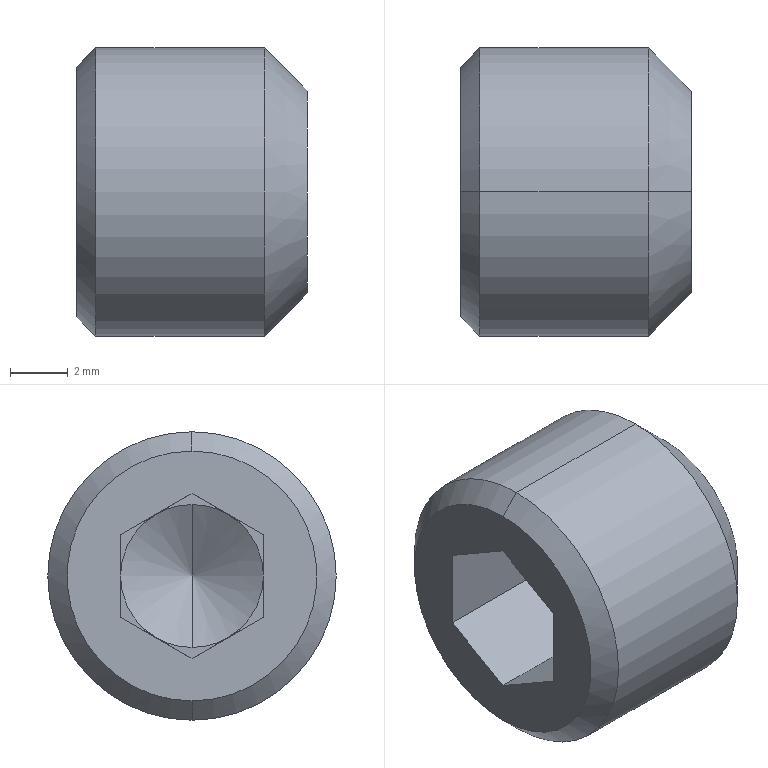Part | STEP file | 1 solid | 22 faces | box 8 x 10 x 10 mm | volume 495.582 mm3 | plane 14 | cone 6 | cylinder 2 | commonest cylinder face diameters 10 x2
STEP:
#1=CARTESIAN_POINT('',(0.,0.,0.));
#2=DIRECTION('',(0.,0.,1.));
#3=DIRECTION('',(1.,0.,0.));
#4=AXIS2_PLACEMENT_3D('',#1,#2,#3);
#5=CARTESIAN_POINT('',(4.,2.477,0.));
#6=VERTEX_POINT('',#5);
#7=CARTESIAN_POINT('',(4.,2.477,-1.43));
#8=VERTEX_POINT('',#7);
#9=CARTESIAN_POINT('',(4.,2.477,-1.43));
#10=DIRECTION('',(0.,0.,-1.));
#11=VECTOR('',#10,1.);
#12=LINE('',#9,#11);
#13=CARTESIAN_POINT('',(4.,-2.477,-1.43));
#14=DIRECTION('',(-1.,0.,0.));
#15=DIRECTION('',(0.,0.,1.));
#16=AXIS2_PLACEMENT_3D('',#13,#14,#15);
#17=PLANE('',#16);
#18=CARTESIAN_POINT('',(0.,4.954));
#19=DIRECTION('',(-1.,0.));
#20=VECTOR('',#19,1.);
#21=LINE('',#18,#20);
#22=(GEOMETRIC_REPRESENTATION_CONTEXT(2)PARAMETRIC_REPRESENTATION_CONTEXT()REPRESENTATION_CONTEXT('',''));
#23=DEFINITIONAL_REPRESENTATION('',(#21),#22);
#24=PCURVE('',#17,#23);
#25=CARTESIAN_POINT('',(4.,2.477,1.43));
#26=DIRECTION('',(0.,1.,0.));
#27=DIRECTION('',(0.,0.,-1.));
#28=AXIS2_PLACEMENT_3D('',#25,#26,#27);
#29=PLANE('',#28);
#30=CARTESIAN_POINT('',(2.86,0.));
#31=DIRECTION('',(1.,0.));
#32=VECTOR('',#31,1.);
#33=LINE('',#30,#32);
#34=(GEOMETRIC_REPRESENTATION_CONTEXT(2)PARAMETRIC_REPRESENTATION_CONTEXT()REPRESENTATION_CONTEXT('',''));
#35=DEFINITIONAL_REPRESENTATION('',(#33),#34);
#36=PCURVE('',#29,#35);
#37=SURFACE_CURVE('',#12,(#24,#36),.PCURVE_S1.);
#38=EDGE_CURVE('',#6,#8,#37,.T.);
#39=ORIENTED_EDGE('',*,*,#38,.T.);
#40=CARTESIAN_POINT('',(4.,1.238,-2.145));
#41=VERTEX_POINT('',#40);
#42=CARTESIAN_POINT('',(4.,2.477,-1.43));
#43=DIRECTION('',(0.,-0.866,-0.5));
#44=VECTOR('',#43,1.);
#45=LINE('',#42,#44);
#46=CARTESIAN_POINT('',(0.,4.954));
#47=DIRECTION('',(-0.5,-0.866));
#48=VECTOR('',#47,1.);
#49=LINE('',#46,#48);
#50=(GEOMETRIC_REPRESENTATION_CONTEXT(2)PARAMETRIC_REPRESENTATION_CONTEXT()REPRESENTATION_CONTEXT('',''));
#51=DEFINITIONAL_REPRESENTATION('',(#49),#50);
#52=PCURVE('',#17,#51);
#53=CARTESIAN_POINT('',(4.,2.477,-1.43));
#54=DIRECTION('',(0.,0.5,-0.866));
#55=DIRECTION('',(-1.,0.,0.));
#56=AXIS2_PLACEMENT_3D('',#53,#54,#55);
#57=PLANE('',#56);
#58=CARTESIAN_POINT('',(0.,0.));
#59=DIRECTION('',(0.,-1.));
#60=VECTOR('',#59,1.);
#61=LINE('',#58,#60);
#62=(GEOMETRIC_REPRESENTATION_CONTEXT(2)PARAMETRIC_REPRESENTATION_CONTEXT()REPRESENTATION_CONTEXT('',''));
#63=DEFINITIONAL_REPRESENTATION('',(#61),#62);
#64=PCURVE('',#57,#63);
#65=SURFACE_CURVE('',#45,(#52,#64),.PCURVE_S1.);
#66=EDGE_CURVE('',#8,#41,#65,.T.);
#67=ORIENTED_EDGE('',*,*,#66,.T.);
#68=CARTESIAN_POINT('',(4.,0.,0.));
#69=DIRECTION('',(1.,0.,0.));
#70=DIRECTION('',(0.,0.,1.));
#71=AXIS2_PLACEMENT_3D('',#68,#69,#70);
#72=CIRCLE('',#71,2.477);
#73=CARTESIAN_POINT('',(3.907,2.477));
#74=CARTESIAN_POINT('',(3.907,-1.813));
#75=CARTESIAN_POINT('',(0.1916,0.3318));
#76=CARTESIAN_POINT('',(-3.524,2.477));
#77=CARTESIAN_POINT('',(0.1916,4.622));
#78=CARTESIAN_POINT('',(3.907,6.767));
#79=CARTESIAN_POINT('',(3.907,2.477));
#80=(BOUNDED_CURVE()B_SPLINE_CURVE(2,(#73,#74,#75,#76,#77,#78,#79),.UNSPECIFIED.,.T.,.F.)B_SPLINE_CURVE_WITH_KNOTS((1,2,2,2,2,1),(-2.094,0.,2.094,4.189,6.283,8.378),.UNSPECIFIED.)CURVE()GEOMETRIC_REPRESENTATION_ITEM()RATIONAL_B_SPLINE_CURVE((1.,0.5,1.,0.5,1.,0.5,1.))REPRESENTATION_ITEM(''));
#81=(GEOMETRIC_REPRESENTATION_CONTEXT(2)PARAMETRIC_REPRESENTATION_CONTEXT()REPRESENTATION_CONTEXT('',''));
#82=DEFINITIONAL_REPRESENTATION('',(#80),#81);
#83=PCURVE('',#17,#82);
#84=CARTESIAN_POINT('',(4.,0.,0.));
#85=DIRECTION('',(-1.,0.,0.));
#86=DIRECTION('',(0.,0.,1.));
#87=AXIS2_PLACEMENT_3D('',#84,#85,#86);
#88=CONICAL_SURFACE('',#87,2.477,1.047);
#89=CARTESIAN_POINT('',(6.283,0.));
#90=DIRECTION('',(-1.,0.));
#91=VECTOR('',#90,1.);
#92=LINE('',#89,#91);
#93=(GEOMETRIC_REPRESENTATION_CONTEXT(2)PARAMETRIC_REPRESENTATION_CONTEXT()REPRESENTATION_CONTEXT('',''));
#94=DEFINITIONAL_REPRESENTATION('',(#92),#93);
#95=PCURVE('',#88,#94);
#96=SURFACE_CURVE('',#72,(#83,#95),.PCURVE_S1.);
#97=EDGE_CURVE('',#41,#6,#96,.T.);
#98=ORIENTED_EDGE('',*,*,#97,.T.);
#99=EDGE_LOOP('',(#39,#67,#98));
#100=FACE_BOUND('',#99,.T.);
#101=ADVANCED_FACE('',(#100),#17,.T.);
#102=CARTESIAN_POINT('',(4.,1.238,2.145));
#103=VERTEX_POINT('',#102);
#104=CARTESIAN_POINT('',(4.,2.477,1.43));
#105=VERTEX_POINT('',#104);
#106=CARTESIAN_POINT('',(4.,1.238,2.145));
#107=DIRECTION('',(0.,0.866,-0.5));
#108=VECTOR('',#107,1.);
#109=LINE('',#106,#108);
#110=CARTESIAN_POINT('',(4.,-2.477,-1.43));
#111=DIRECTION('',(-1.,0.,0.));
#112=DIRECTION('',(0.,0.,1.));
#113=AXIS2_PLACEMENT_3D('',#110,#111,#112);
#114=PLANE('',#113);
#115=CARTESIAN_POINT('',(3.575,3.715));
#116=DIRECTION('',(-0.5,0.866));
#117=VECTOR('',#116,1.);
#118=LINE('',#115,#117);
#119=(GEOMETRIC_REPRESENTATION_CONTEXT(2)PARAMETRIC_REPRESENTATION_CONTEXT()REPRESENTATION_CONTEXT('',''));
#120=DEFINITIONAL_REPRESENTATION('',(#118),#119);
#121=PCURVE('',#114,#120);
#122=CARTESIAN_POINT('',(4.,0.,2.86));
#123=DIRECTION('',(0.,0.5,0.866));
#124=DIRECTION('',(1.,0.,0.));
#125=AXIS2_PLACEMENT_3D('',#122,#123,#124);
#126=PLANE('',#125);
#127=CARTESIAN_POINT('',(0.,1.43));
#128=DIRECTION('',(0.,1.));
#129=VECTOR('',#128,1.);
#130=LINE('',#127,#129);
#131=(GEOMETRIC_REPRESENTATION_CONTEXT(2)PARAMETRIC_REPRESENTATION_CONTEXT()REPRESENTATION_CONTEXT('',''));
#132=DEFINITIONAL_REPRESENTATION('',(#130),#131);
#133=PCURVE('',#126,#132);
#134=SURFACE_CURVE('',#109,(#121,#133),.PCURVE_S1.);
#135=EDGE_CURVE('',#103,#105,#134,.T.);
#136=ORIENTED_EDGE('',*,*,#135,.T.);
#137=CARTESIAN_POINT('',(4.,2.477,-1.43));
#138=DIRECTION('',(0.,0.,-1.));
#139=VECTOR('',#138,1.);
#140=LINE('',#137,#139);
#141=CARTESIAN_POINT('',(0.,4.954));
#142=DIRECTION('',(-1.,0.));
#143=VECTOR('',#142,1.);
#144=LINE('',#141,#143);
#145=(GEOMETRIC_REPRESENTATION_CONTEXT(2)PARAMETRIC_REPRESENTATION_CONTEXT()REPRESENTATION_CONTEXT('',''));
#146=DEFINITIONAL_REPRESENTATION('',(#144),#145);
#147=PCURVE('',#114,#146);
#148=CARTESIAN_POINT('',(2.86,0.));
#149=DIRECTION('',(1.,0.));
#150=VECTOR('',#149,1.);
#151=LINE('',#148,#150);
#152=(GEOMETRIC_REPRESENTATION_CONTEXT(2)PARAMETRIC_REPRESENTATION_CONTEXT()REPRESENTATION_CONTEXT('',''));
#153=DEFINITIONAL_REPRESENTATION('',(#151),#152);
#154=PCURVE('',#29,#153);
#155=SURFACE_CURVE('',#140,(#147,#154),.PCURVE_S1.);
#156=EDGE_CURVE('',#105,#6,#155,.T.);
#157=ORIENTED_EDGE('',*,*,#156,.T.);
#158=CARTESIAN_POINT('',(4.,0.,0.));
#159=DIRECTION('',(1.,0.,0.));
#160=DIRECTION('',(0.,0.,1.));
#161=AXIS2_PLACEMENT_3D('',#158,#159,#160);
#162=CIRCLE('',#161,2.477);
#163=CARTESIAN_POINT('',(3.907,2.477));
#164=CARTESIAN_POINT('',(3.907,-1.813));
#165=CARTESIAN_POINT('',(0.1916,0.3318));
#166=CARTESIAN_POINT('',(-3.524,2.477));
#167=CARTESIAN_POINT('',(0.1916,4.622));
#168=CARTESIAN_POINT('',(3.907,6.767));
#169=CARTESIAN_POINT('',(3.907,2.477));
#170=(BOUNDED_CURVE()B_SPLINE_CURVE(2,(#163,#164,#165,#166,#167,#168,#169),.UNSPECIFIED.,.T.,.F.)B_SPLINE_CURVE_WITH_KNOTS((1,2,2,2,2,1),(-2.094,0.,2.094,4.189,6.283,8.378),.UNSPECIFIED.)CURVE()GEOMETRIC_REPRESENTATION_ITEM()RATIONAL_B_SPLINE_CURVE((1.,0.5,1.,0.5,1.,0.5,1.))REPRESENTATION_ITEM(''));
#171=(GEOMETRIC_REPRESENTATION_CONTEXT(2)PARAMETRIC_REPRESENTATION_CONTEXT()REPRESENTATION_CONTEXT('',''));
#172=DEFINITIONAL_REPRESENTATION('',(#170),#171);
#173=PCURVE('',#114,#172);
#174=CARTESIAN_POINT('',(6.283,0.));
#175=DIRECTION('',(-1.,0.));
#176=VECTOR('',#175,1.);
#177=LINE('',#174,#176);
#178=(GEOMETRIC_REPRESENTATION_CONTEXT(2)PARAMETRIC_REPRESENTATION_CONTEXT()REPRESENTATION_CONTEXT('',''));
#179=DEFINITIONAL_REPRESENTATION('',(#177),#178);
#180=PCURVE('',#88,#179);
#181=SURFACE_CURVE('',#162,(#173,#180),.PCURVE_S1.);
#182=EDGE_CURVE('',#6,#103,#181,.T.);
#183=ORIENTED_EDGE('',*,*,#182,.T.);
#184=EDGE_LOOP('',(#136,#157,#183));
#185=FACE_BOUND('',#184,.T.);
#186=ADVANCED_FACE('',(#185),#114,.T.);
#187=CARTESIAN_POINT('',(4.,-1.238,-2.145));
#188=VERTEX_POINT('',#187);
#189=CARTESIAN_POINT('',(4.,-2.477,-1.43));
#190=VERTEX_POINT('',#189);
#191=CARTESIAN_POINT('',(4.,-1.238,-2.145));
#192=DIRECTION('',(0.,-0.866,0.5));
#193=VECTOR('',#192,1.);
#194=LINE('',#191,#193);
#195=CARTESIAN_POINT('',(4.,-2.477,-1.43));
#196=DIRECTION('',(-1.,0.,0.));
#197=DIRECTION('',(0.,0.,1.));
#198=AXIS2_PLACEMENT_3D('',#195,#196,#197);
#199=PLANE('',#198);
#200=CARTESIAN_POINT('',(-0.715,1.238));
#201=DIRECTION('',(0.5,-0.866));
#202=VECTOR('',#201,1.);
#203=LINE('',#200,#202);
#204=(GEOMETRIC_REPRESENTATION_CONTEXT(2)PARAMETRIC_REPRESENTATION_CONTEXT()REPRESENTATION_CONTEXT('',''));
#205=DEFINITIONAL_REPRESENTATION('',(#203),#204);
#206=PCURVE('',#199,#205);
#207=CARTESIAN_POINT('',(4.,0.,-2.86));
#208=DIRECTION('',(0.,-0.5,-0.866));
#209=DIRECTION('',(0.,-0.866,0.5));
#210=AXIS2_PLACEMENT_3D('',#207,#208,#209);
#211=PLANE('',#210);
#212=CARTESIAN_POINT('',(1.43,0.));
#213=DIRECTION('',(1.,0.));
#214=VECTOR('',#213,1.);
#215=LINE('',#212,#214);
#216=(GEOMETRIC_REPRESENTATION_CONTEXT(2)PARAMETRIC_REPRESENTATION_CONTEXT()REPRESENTATION_CONTEXT('',''));
#217=DEFINITIONAL_REPRESENTATION('',(#215),#216);
#218=PCURVE('',#211,#217);
#219=SURFACE_CURVE('',#194,(#206,#218),.PCURVE_S1.);
#220=EDGE_CURVE('',#188,#190,#219,.T.);
#221=ORIENTED_EDGE('',*,*,#220,.T.);
#222=CARTESIAN_POINT('',(4.,-2.477,0.));
#223=VERTEX_POINT('',#222);
#224=CARTESIAN_POINT('',(4.,-2.477,-1.43));
#225=DIRECTION('',(0.,0.,1.));
#226=VECTOR('',#225,1.);
#227=LINE('',#224,#226);
#228=CARTESIAN_POINT('',(0.,0.));
#229=DIRECTION('',(1.,0.));
#230=VECTOR('',#229,1.);
#231=LINE('',#228,#230);
#232=(GEOMETRIC_REPRESENTATION_CONTEXT(2)PARAMETRIC_REPRESENTATION_CONTEXT()REPRESENTATION_CONTEXT('',''));
#233=DEFINITIONAL_REPRESENTATION('',(#231),#232);
#234=PCURVE('',#199,#233);
#235=CARTESIAN_POINT('',(4.,-2.477,-1.43));
#236=DIRECTION('',(0.,-1.,0.));
#237=DIRECTION('',(-1.,0.,0.));
#238=AXIS2_PLACEMENT_3D('',#235,#236,#237);
#239=PLANE('',#238);
#240=CARTESIAN_POINT('',(0.,0.));
#241=DIRECTION('',(0.,-1.));
#242=VECTOR('',#241,1.);
#243=LINE('',#240,#242);
#244=(GEOMETRIC_REPRESENTATION_CONTEXT(2)PARAMETRIC_REPRESENTATION_CONTEXT()REPRESENTATION_CONTEXT('',''));
#245=DEFINITIONAL_REPRESENTATION('',(#243),#244);
#246=PCURVE('',#239,#245);
#247=SURFACE_CURVE('',#227,(#234,#246),.PCURVE_S1.);
#248=EDGE_CURVE('',#190,#223,#247,.T.);
#249=ORIENTED_EDGE('',*,*,#248,.T.);
#250=CARTESIAN_POINT('',(4.,0.,0.));
#251=DIRECTION('',(1.,0.,0.));
#252=DIRECTION('',(0.,0.,1.));
#253=AXIS2_PLACEMENT_3D('',#250,#251,#252);
#254=CIRCLE('',#253,2.477);
#255=CARTESIAN_POINT('',(3.907,2.477));
#256=CARTESIAN_POINT('',(3.907,-1.813));
#257=CARTESIAN_POINT('',(0.1916,0.3318));
#258=CARTESIAN_POINT('',(-3.524,2.477));
#259=CARTESIAN_POINT('',(0.1916,4.622));
#260=CARTESIAN_POINT('',(3.907,6.767));
#261=CARTESIAN_POINT('',(3.907,2.477));
#262=(BOUNDED_CURVE()B_SPLINE_CURVE(2,(#255,#256,#257,#258,#259,#260,#261),.UNSPECIFIED.,.T.,.F.)B_SPLINE_CURVE_WITH_KNOTS((1,2,2,2,2,1),(-2.094,0.,2.094,4.189,6.283,8.378),.UNSPECIFIED.)CURVE()GEOMETRIC_REPRESENTATION_ITEM()RATIONAL_B_SPLINE_CURVE((1.,0.5,1.,0.5,1.,0.5,1.))REPRESENTATION_ITEM(''));
#263=(GEOMETRIC_REPRESENTATION_CONTEXT(2)PARAMETRIC_REPRESENTATION_CONTEXT()REPRESENTATION_CONTEXT('',''));
#264=DEFINITIONAL_REPRESENTATION('',(#262),#263);
#265=PCURVE('',#199,#264);
#266=CARTESIAN_POINT('',(4.,0.,0.));
#267=DIRECTION('',(-1.,0.,0.));
#268=DIRECTION('',(0.,0.,1.));
#269=AXIS2_PLACEMENT_3D('',#266,#267,#268);
#270=CONICAL_SURFACE('',#269,2.477,1.047);
#271=CARTESIAN_POINT('',(6.283,0.));
#272=DIRECTION('',(-1.,0.));
#273=VECTOR('',#272,1.);
#274=LINE('',#271,#273);
#275=(GEOMETRIC_REPRESENTATION_CONTEXT(2)PARAMETRIC_REPRESENTATION_CONTEXT()REPRESENTATION_CONTEXT('',''));
#276=DEFINITIONAL_REPRESENTATION('',(#274),#275);
#277=PCURVE('',#270,#276);
#278=SURFACE_CURVE('',#254,(#265,#277),.PCURVE_S1.);
#279=EDGE_CURVE('',#223,#188,#278,.T.);
#280=ORIENTED_EDGE('',*,*,#279,.T.);
#281=EDGE_LOOP('',(#221,#249,#280));
#282=FACE_BOUND('',#281,.T.);
#283=ADVANCED_FACE('',(#282),#199,.T.);
#284=CARTESIAN_POINT('',(4.,0.,-2.477));
#285=VERTEX_POINT('',#284);
#286=CARTESIAN_POINT('',(4.,0.,0.));
#287=DIRECTION('',(1.,0.,0.));
#288=DIRECTION('',(0.,0.,1.));
#289=AXIS2_PLACEMENT_3D('',#286,#287,#288);
#290=CIRCLE('',#289,2.477);
#291=CARTESIAN_POINT('',(6.283,0.));
#292=DIRECTION('',(-1.,0.));
#293=VECTOR('',#292,1.);
#294=LINE('',#291,#293);
#295=(GEOMETRIC_REPRESENTATION_CONTEXT(2)PARAMETRIC_REPRESENTATION_CONTEXT()REPRESENTATION_CONTEXT('',''));
#296=DEFINITIONAL_REPRESENTATION('',(#294),#295);
#297=PCURVE('',#88,#296);
#298=CARTESIAN_POINT('',(4.,-2.477,-1.43));
#299=DIRECTION('',(-1.,0.,0.));
#300=DIRECTION('',(0.,0.,1.));
#301=AXIS2_PLACEMENT_3D('',#298,#299,#300);
#302=PLANE('',#301);
#303=CARTESIAN_POINT('',(3.907,2.477));
#304=CARTESIAN_POINT('',(3.907,-1.813));
#305=CARTESIAN_POINT('',(0.1916,0.3318));
#306=CARTESIAN_POINT('',(-3.524,2.477));
#307=CARTESIAN_POINT('',(0.1916,4.622));
#308=CARTESIAN_POINT('',(3.907,6.767));
#309=CARTESIAN_POINT('',(3.907,2.477));
#310=(BOUNDED_CURVE()B_SPLINE_CURVE(2,(#303,#304,#305,#306,#307,#308,#309),.UNSPECIFIED.,.T.,.F.)B_SPLINE_CURVE_WITH_KNOTS((1,2,2,2,2,1),(-2.094,0.,2.094,4.189,6.283,8.378),.UNSPECIFIED.)CURVE()GEOMETRIC_REPRESENTATION_ITEM()RATIONAL_B_SPLINE_CURVE((1.,0.5,1.,0.5,1.,0.5,1.))REPRESENTATION_ITEM(''));
#311=(GEOMETRIC_REPRESENTATION_CONTEXT(2)PARAMETRIC_REPRESENTATION_CONTEXT()REPRESENTATION_CONTEXT('',''));
#312=DEFINITIONAL_REPRESENTATION('',(#310),#311);
#313=PCURVE('',#302,#312);
#314=SURFACE_CURVE('',#290,(#297,#313),.PCURVE_S1.);
#315=EDGE_CURVE('',#285,#41,#314,.T.);
#316=ORIENTED_EDGE('',*,*,#315,.T.);
#317=ORIENTED_EDGE('',*,*,#97,.T.);
#318=ORIENTED_EDGE('',*,*,#182,.T.);
#319=CARTESIAN_POINT('',(4.,0.,2.477));
#320=VERTEX_POINT('',#319);
#321=CARTESIAN_POINT('',(4.,0.,0.));
#322=DIRECTION('',(1.,0.,0.));
#323=DIRECTION('',(0.,0.,1.));
#324=AXIS2_PLACEMENT_3D('',#321,#322,#323);
#325=CIRCLE('',#324,2.477);
#326=CARTESIAN_POINT('',(6.283,0.));
#327=DIRECTION('',(-1.,0.));
#328=VECTOR('',#327,1.);
#329=LINE('',#326,#328);
#330=(GEOMETRIC_REPRESENTATION_CONTEXT(2)PARAMETRIC_REPRESENTATION_CONTEXT()REPRESENTATION_CONTEXT('',''));
#331=DEFINITIONAL_REPRESENTATION('',(#329),#330);
#332=PCURVE('',#88,#331);
#333=CARTESIAN_POINT('',(4.,-2.477,-1.43));
#334=DIRECTION('',(-1.,0.,0.));
#335=DIRECTION('',(0.,0.,1.));
#336=AXIS2_PLACEMENT_3D('',#333,#334,#335);
#337=PLANE('',#336);
#338=CARTESIAN_POINT('',(3.907,2.477));
#339=CARTESIAN_POINT('',(3.907,-1.813));
#340=CARTESIAN_POINT('',(0.1916,0.3318));
#341=CARTESIAN_POINT('',(-3.524,2.477));
#342=CARTESIAN_POINT('',(0.1916,4.622));
#343=CARTESIAN_POINT('',(3.907,6.767));
#344=CARTESIAN_POINT('',(3.907,2.477));
#345=(BOUNDED_CURVE()B_SPLINE_CURVE(2,(#338,#339,#340,#341,#342,#343,#344),.UNSPECIFIED.,.T.,.F.)B_SPLINE_CURVE_WITH_KNOTS((1,2,2,2,2,1),(-2.094,0.,2.094,4.189,6.283,8.378),.UNSPECIFIED.)CURVE()GEOMETRIC_REPRESENTATION_ITEM()RATIONAL_B_SPLINE_CURVE((1.,0.5,1.,0.5,1.,0.5,1.))REPRESENTATION_ITEM(''));
#346=(GEOMETRIC_REPRESENTATION_CONTEXT(2)PARAMETRIC_REPRESENTATION_CONTEXT()REPRESENTATION_CONTEXT('',''));
#347=DEFINITIONAL_REPRESENTATION('',(#345),#346);
#348=PCURVE('',#337,#347);
#349=SURFACE_CURVE('',#325,(#332,#348),.PCURVE_S1.);
#350=EDGE_CURVE('',#103,#320,#349,.T.);
#351=ORIENTED_EDGE('',*,*,#350,.T.);
#352=CARTESIAN_POINT('',(5.43,0.,0.));
#353=VERTEX_POINT('',#352);
#354=CARTESIAN_POINT('',(4.,0.,2.477));
#355=DIRECTION('',(-0.5,0.,0.866));
#356=VECTOR('',#355,1.);
#357=LINE('',#354,#356);
#358=CARTESIAN_POINT('',(0.,0.));
#359=DIRECTION('',(0.,1.));
#360=VECTOR('',#359,1.);
#361=LINE('',#358,#360);
#362=(GEOMETRIC_REPRESENTATION_CONTEXT(2)PARAMETRIC_REPRESENTATION_CONTEXT()REPRESENTATION_CONTEXT('',''));
#363=DEFINITIONAL_REPRESENTATION('',(#361),#362);
#364=PCURVE('',#88,#363);
#365=CARTESIAN_POINT('',(6.283,0.));
#366=DIRECTION('',(0.,1.));
#367=VECTOR('',#366,1.);
#368=LINE('',#365,#367);
#369=(GEOMETRIC_REPRESENTATION_CONTEXT(2)PARAMETRIC_REPRESENTATION_CONTEXT()REPRESENTATION_CONTEXT('',''));
#370=DEFINITIONAL_REPRESENTATION('',(#368),#369);
#371=PCURVE('',#270,#370);
#372=SURFACE_CURVE('',#357,(#364,#371),.PCURVE_S1.);
#373=EDGE_CURVE('',#353,#320,#372,.T.);
#374=ORIENTED_EDGE('',*,*,#373,.F.);
#375=CARTESIAN_POINT('',(4.,0.,-2.477));
#376=DIRECTION('',(-0.5,0.,-0.866));
#377=VECTOR('',#376,1.);
#378=LINE('',#375,#377);
#379=CARTESIAN_POINT('',(3.142,0.));
#380=DIRECTION('',(0.,1.));
#381=VECTOR('',#380,1.);
#382=LINE('',#379,#381);
#383=(GEOMETRIC_REPRESENTATION_CONTEXT(2)PARAMETRIC_REPRESENTATION_CONTEXT()REPRESENTATION_CONTEXT('',''));
#384=DEFINITIONAL_REPRESENTATION('',(#382),#383);
#385=PCURVE('',#88,#384);
#386=CARTESIAN_POINT('',(3.142,0.));
#387=DIRECTION('',(0.,1.));
#388=VECTOR('',#387,1.);
#389=LINE('',#386,#388);
#390=(GEOMETRIC_REPRESENTATION_CONTEXT(2)PARAMETRIC_REPRESENTATION_CONTEXT()REPRESENTATION_CONTEXT('',''));
#391=DEFINITIONAL_REPRESENTATION('',(#389),#390);
#392=PCURVE('',#270,#391);
#393=SURFACE_CURVE('',#378,(#385,#392),.PCURVE_S1.);
#394=EDGE_CURVE('',#353,#285,#393,.T.);
#395=ORIENTED_EDGE('',*,*,#394,.T.);
#396=EDGE_LOOP('',(#316,#317,#318,#351,#374,#395));
#397=FACE_BOUND('',#396,.F.);
#398=ADVANCED_FACE('',(#397),#88,.F.);
#399=CARTESIAN_POINT('',(4.,-2.477,1.43));
#400=VERTEX_POINT('',#399);
#401=CARTESIAN_POINT('',(4.,-2.477,-1.43));
#402=DIRECTION('',(0.,0.,1.));
#403=VECTOR('',#402,1.);
#404=LINE('',#401,#403);
#405=CARTESIAN_POINT('',(4.,-2.477,-1.43));
#406=DIRECTION('',(-1.,0.,0.));
#407=DIRECTION('',(0.,0.,1.));
#408=AXIS2_PLACEMENT_3D('',#405,#406,#407);
#409=PLANE('',#408);
#410=CARTESIAN_POINT('',(0.,0.));
#411=DIRECTION('',(1.,0.));
#412=VECTOR('',#411,1.);
#413=LINE('',#410,#412);
#414=(GEOMETRIC_REPRESENTATION_CONTEXT(2)PARAMETRIC_REPRESENTATION_CONTEXT()REPRESENTATION_CONTEXT('',''));
#415=DEFINITIONAL_REPRESENTATION('',(#413),#414);
#416=PCURVE('',#409,#415);
#417=CARTESIAN_POINT('',(0.,0.));
#418=DIRECTION('',(0.,-1.));
#419=VECTOR('',#418,1.);
#420=LINE('',#417,#419);
#421=(GEOMETRIC_REPRESENTATION_CONTEXT(2)PARAMETRIC_REPRESENTATION_CONTEXT()REPRESENTATION_CONTEXT('',''));
#422=DEFINITIONAL_REPRESENTATION('',(#420),#421);
#423=PCURVE('',#239,#422);
#424=SURFACE_CURVE('',#404,(#416,#423),.PCURVE_S1.);
#425=EDGE_CURVE('',#223,#400,#424,.T.);
#426=ORIENTED_EDGE('',*,*,#425,.T.);
#427=CARTESIAN_POINT('',(4.,-1.238,2.145));
#428=VERTEX_POINT('',#427);
#429=CARTESIAN_POINT('',(4.,-2.477,1.43));
#430=DIRECTION('',(0.,0.866,0.5));
#431=VECTOR('',#430,1.);
#432=LINE('',#429,#431);
#433=CARTESIAN_POINT('',(2.86,0.));
#434=DIRECTION('',(0.5,0.866));
#435=VECTOR('',#434,1.);
#436=LINE('',#433,#435);
#437=(GEOMETRIC_REPRESENTATION_CONTEXT(2)PARAMETRIC_REPRESENTATION_CONTEXT()REPRESENTATION_CONTEXT('',''));
#438=DEFINITIONAL_REPRESENTATION('',(#436),#437);
#439=PCURVE('',#409,#438);
#440=CARTESIAN_POINT('',(4.,-2.477,1.43));
#441=DIRECTION('',(0.,-0.5,0.866));
#442=DIRECTION('',(-1.,0.,0.));
#443=AXIS2_PLACEMENT_3D('',#440,#441,#442);
#444=PLANE('',#443);
#445=CARTESIAN_POINT('',(0.,0.));
#446=DIRECTION('',(0.,-1.));
#447=VECTOR('',#446,1.);
#448=LINE('',#445,#447);
#449=(GEOMETRIC_REPRESENTATION_CONTEXT(2)PARAMETRIC_REPRESENTATION_CONTEXT()REPRESENTATION_CONTEXT('',''));
#450=DEFINITIONAL_REPRESENTATION('',(#448),#449);
#451=PCURVE('',#444,#450);
#452=SURFACE_CURVE('',#432,(#439,#451),.PCURVE_S1.);
#453=EDGE_CURVE('',#400,#428,#452,.T.);
#454=ORIENTED_EDGE('',*,*,#453,.T.);
#455=CARTESIAN_POINT('',(4.,0.,0.));
#456=DIRECTION('',(1.,0.,0.));
#457=DIRECTION('',(0.,0.,1.));
#458=AXIS2_PLACEMENT_3D('',#455,#456,#457);
#459=CIRCLE('',#458,2.477);
#460=CARTESIAN_POINT('',(3.907,2.477));
#461=CARTESIAN_POINT('',(3.907,-1.813));
#462=CARTESIAN_POINT('',(0.1916,0.3318));
#463=CARTESIAN_POINT('',(-3.524,2.477));
#464=CARTESIAN_POINT('',(0.1916,4.622));
#465=CARTESIAN_POINT('',(3.907,6.767));
#466=CARTESIAN_POINT('',(3.907,2.477));
#467=(BOUNDED_CURVE()B_SPLINE_CURVE(2,(#460,#461,#462,#463,#464,#465,#466),.UNSPECIFIED.,.T.,.F.)B_SPLINE_CURVE_WITH_KNOTS((1,2,2,2,2,1),(-2.094,0.,2.094,4.189,6.283,8.378),.UNSPECIFIED.)CURVE()GEOMETRIC_REPRESENTATION_ITEM()RATIONAL_B_SPLINE_CURVE((1.,0.5,1.,0.5,1.,0.5,1.))REPRESENTATION_ITEM(''));
#468=(GEOMETRIC_REPRESENTATION_CONTEXT(2)PARAMETRIC_REPRESENTATION_CONTEXT()REPRESENTATION_CONTEXT('',''));
#469=DEFINITIONAL_REPRESENTATION('',(#467),#468);
#470=PCURVE('',#409,#469);
#471=CARTESIAN_POINT('',(6.283,0.));
#472=DIRECTION('',(-1.,0.));
#473=VECTOR('',#472,1.);
#474=LINE('',#471,#473);
#475=(GEOMETRIC_REPRESENTATION_CONTEXT(2)PARAMETRIC_REPRESENTATION_CONTEXT()REPRESENTATION_CONTEXT('',''));
#476=DEFINITIONAL_REPRESENTATION('',(#474),#475);
#477=PCURVE('',#270,#476);
#478=SURFACE_CURVE('',#459,(#470,#477),.PCURVE_S1.);
#479=EDGE_CURVE('',#428,#223,#478,.T.);
#480=ORIENTED_EDGE('',*,*,#479,.T.);
#481=EDGE_LOOP('',(#426,#454,#480));
#482=FACE_BOUND('',#481,.T.);
#483=ADVANCED_FACE('',(#482),#409,.T.);
#484=CARTESIAN_POINT('',(4.,0.,2.86));
#485=VERTEX_POINT('',#484);
#486=CARTESIAN_POINT('',(4.,0.,2.86));
#487=DIRECTION('',(0.,0.866,-0.5));
#488=VECTOR('',#487,1.);
#489=LINE('',#486,#488);
#490=CARTESIAN_POINT('',(4.29,2.477));
#491=DIRECTION('',(-0.5,0.866));
#492=VECTOR('',#491,1.);
#493=LINE('',#490,#492);
#494=(GEOMETRIC_REPRESENTATION_CONTEXT(2)PARAMETRIC_REPRESENTATION_CONTEXT()REPRESENTATION_CONTEXT('',''));
#495=DEFINITIONAL_REPRESENTATION('',(#493),#494);
#496=PCURVE('',#337,#495);
#497=CARTESIAN_POINT('',(0.,0.));
#498=DIRECTION('',(0.,1.));
#499=VECTOR('',#498,1.);
#500=LINE('',#497,#499);
#501=(GEOMETRIC_REPRESENTATION_CONTEXT(2)PARAMETRIC_REPRESENTATION_CONTEXT()REPRESENTATION_CONTEXT('',''));
#502=DEFINITIONAL_REPRESENTATION('',(#500),#501);
#503=PCURVE('',#126,#502);
#504=SURFACE_CURVE('',#489,(#496,#503),.PCURVE_S1.);
#505=EDGE_CURVE('',#485,#103,#504,.T.);
#506=ORIENTED_EDGE('',*,*,#505,.T.);
#507=ORIENTED_EDGE('',*,*,#350,.T.);
#508=CARTESIAN_POINT('',(4.,0.,0.));
#509=DIRECTION('',(1.,0.,0.));
#510=DIRECTION('',(0.,0.,1.));
#511=AXIS2_PLACEMENT_3D('',#508,#509,#510);
#512=CIRCLE('',#511,2.477);
#513=CARTESIAN_POINT('',(3.907,2.477));
#514=CARTESIAN_POINT('',(3.907,-1.813));
#515=CARTESIAN_POINT('',(0.1916,0.3318));
#516=CARTESIAN_POINT('',(-3.524,2.477));
#517=CARTESIAN_POINT('',(0.1916,4.622));
#518=CARTESIAN_POINT('',(3.907,6.767));
#519=CARTESIAN_POINT('',(3.907,2.477));
#520=(BOUNDED_CURVE()B_SPLINE_CURVE(2,(#513,#514,#515,#516,#517,#518,#519),.UNSPECIFIED.,.T.,.F.)B_SPLINE_CURVE_WITH_KNOTS((1,2,2,2,2,1),(-2.094,0.,2.094,4.189,6.283,8.378),.UNSPECIFIED.)CURVE()GEOMETRIC_REPRESENTATION_ITEM()RATIONAL_B_SPLINE_CURVE((1.,0.5,1.,0.5,1.,0.5,1.))REPRESENTATION_ITEM(''));
#521=(GEOMETRIC_REPRESENTATION_CONTEXT(2)PARAMETRIC_REPRESENTATION_CONTEXT()REPRESENTATION_CONTEXT('',''));
#522=DEFINITIONAL_REPRESENTATION('',(#520),#521);
#523=PCURVE('',#337,#522);
#524=CARTESIAN_POINT('',(6.283,0.));
#525=DIRECTION('',(-1.,0.));
#526=VECTOR('',#525,1.);
#527=LINE('',#524,#526);
#528=(GEOMETRIC_REPRESENTATION_CONTEXT(2)PARAMETRIC_REPRESENTATION_CONTEXT()REPRESENTATION_CONTEXT('',''));
#529=DEFINITIONAL_REPRESENTATION('',(#527),#528);
#530=PCURVE('',#270,#529);
#531=SURFACE_CURVE('',#512,(#523,#530),.PCURVE_S1.);
#532=EDGE_CURVE('',#320,#428,#531,.T.);
#533=ORIENTED_EDGE('',*,*,#532,.T.);
#534=CARTESIAN_POINT('',(4.,-2.477,1.43));
#535=DIRECTION('',(0.,0.866,0.5));
#536=VECTOR('',#535,1.);
#537=LINE('',#534,#536);
#538=CARTESIAN_POINT('',(2.86,0.));
#539=DIRECTION('',(0.5,0.866));
#540=VECTOR('',#539,1.);
#541=LINE('',#538,#540);
#542=(GEOMETRIC_REPRESENTATION_CONTEXT(2)PARAMETRIC_REPRESENTATION_CONTEXT()REPRESENTATION_CONTEXT('',''));
#543=DEFINITIONAL_REPRESENTATION('',(#541),#542);
#544=PCURVE('',#337,#543);
#545=CARTESIAN_POINT('',(0.,0.));
#546=DIRECTION('',(0.,-1.));
#547=VECTOR('',#546,1.);
#548=LINE('',#545,#547);
#549=(GEOMETRIC_REPRESENTATION_CONTEXT(2)PARAMETRIC_REPRESENTATION_CONTEXT()REPRESENTATION_CONTEXT('',''));
#550=DEFINITIONAL_REPRESENTATION('',(#548),#549);
#551=PCURVE('',#444,#550);
#552=SURFACE_CURVE('',#537,(#544,#551),.PCURVE_S1.);
#553=EDGE_CURVE('',#428,#485,#552,.T.);
#554=ORIENTED_EDGE('',*,*,#553,.T.);
#555=EDGE_LOOP('',(#506,#507,#533,#554));
#556=FACE_BOUND('',#555,.T.);
#557=ADVANCED_FACE('',(#556),#337,.T.);
#558=CARTESIAN_POINT('',(4.,0.,-2.86));
#559=VERTEX_POINT('',#558);
#560=CARTESIAN_POINT('',(4.,0.,-2.86));
#561=DIRECTION('',(0.,-0.866,0.5));
#562=VECTOR('',#561,1.);
#563=LINE('',#560,#562);
#564=CARTESIAN_POINT('',(-1.43,2.477));
#565=DIRECTION('',(0.5,-0.866));
#566=VECTOR('',#565,1.);
#567=LINE('',#564,#566);
#568=(GEOMETRIC_REPRESENTATION_CONTEXT(2)PARAMETRIC_REPRESENTATION_CONTEXT()REPRESENTATION_CONTEXT('',''));
#569=DEFINITIONAL_REPRESENTATION('',(#567),#568);
#570=PCURVE('',#302,#569);
#571=CARTESIAN_POINT('',(0.,0.));
#572=DIRECTION('',(1.,0.));
#573=VECTOR('',#572,1.);
#574=LINE('',#571,#573);
#575=(GEOMETRIC_REPRESENTATION_CONTEXT(2)PARAMETRIC_REPRESENTATION_CONTEXT()REPRESENTATION_CONTEXT('',''));
#576=DEFINITIONAL_REPRESENTATION('',(#574),#575);
#577=PCURVE('',#211,#576);
#578=SURFACE_CURVE('',#563,(#570,#577),.PCURVE_S1.);
#579=EDGE_CURVE('',#559,#188,#578,.T.);
#580=ORIENTED_EDGE('',*,*,#579,.T.);
#581=CARTESIAN_POINT('',(4.,0.,0.));
#582=DIRECTION('',(1.,0.,0.));
#583=DIRECTION('',(0.,0.,1.));
#584=AXIS2_PLACEMENT_3D('',#581,#582,#583);
#585=CIRCLE('',#584,2.477);
#586=CARTESIAN_POINT('',(3.907,2.477));
#587=CARTESIAN_POINT('',(3.907,-1.813));
#588=CARTESIAN_POINT('',(0.1916,0.3318));
#589=CARTESIAN_POINT('',(-3.524,2.477));
#590=CARTESIAN_POINT('',(0.1916,4.622));
#591=CARTESIAN_POINT('',(3.907,6.767));
#592=CARTESIAN_POINT('',(3.907,2.477));
#593=(BOUNDED_CURVE()B_SPLINE_CURVE(2,(#586,#587,#588,#589,#590,#591,#592),.UNSPECIFIED.,.T.,.F.)B_SPLINE_CURVE_WITH_KNOTS((1,2,2,2,2,1),(-2.094,0.,2.094,4.189,6.283,8.378),.UNSPECIFIED.)CURVE()GEOMETRIC_REPRESENTATION_ITEM()RATIONAL_B_SPLINE_CURVE((1.,0.5,1.,0.5,1.,0.5,1.))REPRESENTATION_ITEM(''));
#594=(GEOMETRIC_REPRESENTATION_CONTEXT(2)PARAMETRIC_REPRESENTATION_CONTEXT()REPRESENTATION_CONTEXT('',''));
#595=DEFINITIONAL_REPRESENTATION('',(#593),#594);
#596=PCURVE('',#302,#595);
#597=CARTESIAN_POINT('',(6.283,0.));
#598=DIRECTION('',(-1.,0.));
#599=VECTOR('',#598,1.);
#600=LINE('',#597,#599);
#601=(GEOMETRIC_REPRESENTATION_CONTEXT(2)PARAMETRIC_REPRESENTATION_CONTEXT()REPRESENTATION_CONTEXT('',''));
#602=DEFINITIONAL_REPRESENTATION('',(#600),#601);
#603=PCURVE('',#270,#602);
#604=SURFACE_CURVE('',#585,(#596,#603),.PCURVE_S1.);
#605=EDGE_CURVE('',#188,#285,#604,.T.);
#606=ORIENTED_EDGE('',*,*,#605,.T.);
#607=ORIENTED_EDGE('',*,*,#315,.T.);
#608=CARTESIAN_POINT('',(4.,2.477,-1.43));
#609=DIRECTION('',(0.,-0.866,-0.5));
#610=VECTOR('',#609,1.);
#611=LINE('',#608,#610);
#612=CARTESIAN_POINT('',(0.,4.954));
#613=DIRECTION('',(-0.5,-0.866));
#614=VECTOR('',#613,1.);
#615=LINE('',#612,#614);
#616=(GEOMETRIC_REPRESENTATION_CONTEXT(2)PARAMETRIC_REPRESENTATION_CONTEXT()REPRESENTATION_CONTEXT('',''));
#617=DEFINITIONAL_REPRESENTATION('',(#615),#616);
#618=PCURVE('',#302,#617);
#619=CARTESIAN_POINT('',(0.,0.));
#620=DIRECTION('',(0.,-1.));
#621=VECTOR('',#620,1.);
#622=LINE('',#619,#621);
#623=(GEOMETRIC_REPRESENTATION_CONTEXT(2)PARAMETRIC_REPRESENTATION_CONTEXT()REPRESENTATION_CONTEXT('',''));
#624=DEFINITIONAL_REPRESENTATION('',(#622),#623);
#625=PCURVE('',#57,#624);
#626=SURFACE_CURVE('',#611,(#618,#625),.PCURVE_S1.);
#627=EDGE_CURVE('',#41,#559,#626,.T.);
#628=ORIENTED_EDGE('',*,*,#627,.T.);
#629=EDGE_LOOP('',(#580,#606,#607,#628));
#630=FACE_BOUND('',#629,.T.);
#631=ADVANCED_FACE('',(#630),#302,.T.);
#632=CARTESIAN_POINT('',(0.,0.,2.86));
#633=VERTEX_POINT('',#632);
#634=CARTESIAN_POINT('',(4.,0.,2.86));
#635=DIRECTION('',(1.,0.,0.));
#636=VECTOR('',#635,1.);
#637=LINE('',#634,#636);
#638=CARTESIAN_POINT('',(0.,-2.86));
#639=DIRECTION('',(-1.,0.));
#640=VECTOR('',#639,1.);
#641=LINE('',#638,#640);
#642=(GEOMETRIC_REPRESENTATION_CONTEXT(2)PARAMETRIC_REPRESENTATION_CONTEXT()REPRESENTATION_CONTEXT('',''));
#643=DEFINITIONAL_REPRESENTATION('',(#641),#642);
#644=PCURVE('',#444,#643);
#645=CARTESIAN_POINT('',(0.,0.));
#646=DIRECTION('',(1.,0.));
#647=VECTOR('',#646,1.);
#648=LINE('',#645,#647);
#649=(GEOMETRIC_REPRESENTATION_CONTEXT(2)PARAMETRIC_REPRESENTATION_CONTEXT()REPRESENTATION_CONTEXT('',''));
#650=DEFINITIONAL_REPRESENTATION('',(#648),#649);
#651=PCURVE('',#126,#650);
#652=SURFACE_CURVE('',#637,(#644,#651),.PCURVE_S1.);
#653=EDGE_CURVE('',#633,#485,#652,.T.);
#654=ORIENTED_EDGE('',*,*,#653,.T.);
#655=ORIENTED_EDGE('',*,*,#553,.F.);
#656=ORIENTED_EDGE('',*,*,#453,.F.);
#657=CARTESIAN_POINT('',(0.,-2.477,1.43));
#658=VERTEX_POINT('',#657);
#659=CARTESIAN_POINT('',(4.,-2.477,1.43));
#660=DIRECTION('',(-1.,0.,0.));
#661=VECTOR('',#660,1.);
#662=LINE('',#659,#661);
#663=CARTESIAN_POINT('',(0.,0.));
#664=DIRECTION('',(1.,0.));
#665=VECTOR('',#664,1.);
#666=LINE('',#663,#665);
#667=(GEOMETRIC_REPRESENTATION_CONTEXT(2)PARAMETRIC_REPRESENTATION_CONTEXT()REPRESENTATION_CONTEXT('',''));
#668=DEFINITIONAL_REPRESENTATION('',(#666),#667);
#669=PCURVE('',#444,#668);
#670=CARTESIAN_POINT('',(0.,-2.86));
#671=DIRECTION('',(1.,0.));
#672=VECTOR('',#671,1.);
#673=LINE('',#670,#672);
#674=(GEOMETRIC_REPRESENTATION_CONTEXT(2)PARAMETRIC_REPRESENTATION_CONTEXT()REPRESENTATION_CONTEXT('',''));
#675=DEFINITIONAL_REPRESENTATION('',(#673),#674);
#676=PCURVE('',#239,#675);
#677=SURFACE_CURVE('',#662,(#669,#676),.PCURVE_S1.);
#678=EDGE_CURVE('',#400,#658,#677,.T.);
#679=ORIENTED_EDGE('',*,*,#678,.T.);
#680=CARTESIAN_POINT('',(0.,-2.477,1.43));
#681=DIRECTION('',(0.,0.866,0.5));
#682=VECTOR('',#681,1.);
#683=LINE('',#680,#682);
#684=CARTESIAN_POINT('',(4.,0.));
#685=DIRECTION('',(0.,-1.));
#686=VECTOR('',#685,1.);
#687=LINE('',#684,#686);
#688=(GEOMETRIC_REPRESENTATION_CONTEXT(2)PARAMETRIC_REPRESENTATION_CONTEXT()REPRESENTATION_CONTEXT('',''));
#689=DEFINITIONAL_REPRESENTATION('',(#687),#688);
#690=PCURVE('',#444,#689);
#691=CARTESIAN_POINT('',(0.,4.33,0.));
#692=DIRECTION('',(1.,0.,0.));
#693=DIRECTION('',(0.,1.,0.));
#694=AXIS2_PLACEMENT_3D('',#691,#692,#693);
#695=PLANE('',#694);
#696=CARTESIAN_POINT('',(-6.807,1.43));
#697=DIRECTION('',(0.866,0.5));
#698=VECTOR('',#697,1.);
#699=LINE('',#696,#698);
#700=(GEOMETRIC_REPRESENTATION_CONTEXT(2)PARAMETRIC_REPRESENTATION_CONTEXT()REPRESENTATION_CONTEXT('',''));
#701=DEFINITIONAL_REPRESENTATION('',(#699),#700);
#702=PCURVE('',#695,#701);
#703=SURFACE_CURVE('',#683,(#690,#702),.PCURVE_S1.);
#704=EDGE_CURVE('',#658,#633,#703,.T.);
#705=ORIENTED_EDGE('',*,*,#704,.T.);
#706=EDGE_LOOP('',(#654,#655,#656,#679,#705));
#707=FACE_BOUND('',#706,.T.);
#708=ADVANCED_FACE('',(#707),#444,.F.);
#709=CARTESIAN_POINT('',(0.,2.477,1.43));
#710=VERTEX_POINT('',#709);
#711=CARTESIAN_POINT('',(4.,2.477,1.43));
#712=DIRECTION('',(1.,0.,0.));
#713=VECTOR('',#712,1.);
#714=LINE('',#711,#713);
#715=CARTESIAN_POINT('',(0.,2.86));
#716=DIRECTION('',(1.,0.));
#717=VECTOR('',#716,1.);
#718=LINE('',#715,#717);
#719=(GEOMETRIC_REPRESENTATION_CONTEXT(2)PARAMETRIC_REPRESENTATION_CONTEXT()REPRESENTATION_CONTEXT('',''));
#720=DEFINITIONAL_REPRESENTATION('',(#718),#719);
#721=PCURVE('',#126,#720);
#722=CARTESIAN_POINT('',(0.,0.));
#723=DIRECTION('',(0.,-1.));
#724=VECTOR('',#723,1.);
#725=LINE('',#722,#724);
#726=(GEOMETRIC_REPRESENTATION_CONTEXT(2)PARAMETRIC_REPRESENTATION_CONTEXT()REPRESENTATION_CONTEXT('',''));
#727=DEFINITIONAL_REPRESENTATION('',(#725),#726);
#728=PCURVE('',#29,#727);
#729=SURFACE_CURVE('',#714,(#721,#728),.PCURVE_S1.);
#730=EDGE_CURVE('',#710,#105,#729,.T.);
#731=ORIENTED_EDGE('',*,*,#730,.T.);
#732=ORIENTED_EDGE('',*,*,#135,.F.);
#733=ORIENTED_EDGE('',*,*,#505,.F.);
#734=ORIENTED_EDGE('',*,*,#653,.F.);
#735=CARTESIAN_POINT('',(0.,0.,2.86));
#736=DIRECTION('',(0.,0.866,-0.5));
#737=VECTOR('',#736,1.);
#738=LINE('',#735,#737);
#739=CARTESIAN_POINT('',(-4.,0.));
#740=DIRECTION('',(0.,1.));
#741=VECTOR('',#740,1.);
#742=LINE('',#739,#741);
#743=(GEOMETRIC_REPRESENTATION_CONTEXT(2)PARAMETRIC_REPRESENTATION_CONTEXT()REPRESENTATION_CONTEXT('',''));
#744=DEFINITIONAL_REPRESENTATION('',(#742),#743);
#745=PCURVE('',#126,#744);
#746=CARTESIAN_POINT('',(-4.33,2.86));
#747=DIRECTION('',(0.866,-0.5));
#748=VECTOR('',#747,1.);
#749=LINE('',#746,#748);
#750=(GEOMETRIC_REPRESENTATION_CONTEXT(2)PARAMETRIC_REPRESENTATION_CONTEXT()REPRESENTATION_CONTEXT('',''));
#751=DEFINITIONAL_REPRESENTATION('',(#749),#750);
#752=PCURVE('',#695,#751);
#753=SURFACE_CURVE('',#738,(#745,#752),.PCURVE_S1.);
#754=EDGE_CURVE('',#633,#710,#753,.T.);
#755=ORIENTED_EDGE('',*,*,#754,.T.);
#756=EDGE_LOOP('',(#731,#732,#733,#734,#755));
#757=FACE_BOUND('',#756,.T.);
#758=ADVANCED_FACE('',(#757),#126,.F.);
#759=CARTESIAN_POINT('',(0.,2.477,-1.43));
#760=VERTEX_POINT('',#759);
#761=CARTESIAN_POINT('',(4.,2.477,-1.43));
#762=DIRECTION('',(1.,0.,0.));
#763=VECTOR('',#762,1.);
#764=LINE('',#761,#763);
#765=CARTESIAN_POINT('',(2.86,0.));
#766=DIRECTION('',(0.,-1.));
#767=VECTOR('',#766,1.);
#768=LINE('',#765,#767);
#769=(GEOMETRIC_REPRESENTATION_CONTEXT(2)PARAMETRIC_REPRESENTATION_CONTEXT()REPRESENTATION_CONTEXT('',''));
#770=DEFINITIONAL_REPRESENTATION('',(#768),#769);
#771=PCURVE('',#29,#770);
#772=CARTESIAN_POINT('',(0.,0.));
#773=DIRECTION('',(-1.,0.));
#774=VECTOR('',#773,1.);
#775=LINE('',#772,#774);
#776=(GEOMETRIC_REPRESENTATION_CONTEXT(2)PARAMETRIC_REPRESENTATION_CONTEXT()REPRESENTATION_CONTEXT('',''));
#777=DEFINITIONAL_REPRESENTATION('',(#775),#776);
#778=PCURVE('',#57,#777);
#779=SURFACE_CURVE('',#764,(#771,#778),.PCURVE_S1.);
#780=EDGE_CURVE('',#760,#8,#779,.T.);
#781=ORIENTED_EDGE('',*,*,#780,.T.);
#782=ORIENTED_EDGE('',*,*,#38,.F.);
#783=ORIENTED_EDGE('',*,*,#156,.F.);
#784=ORIENTED_EDGE('',*,*,#730,.F.);
#785=CARTESIAN_POINT('',(0.,2.477,0.));
#786=DIRECTION('',(0.,0.,-1.));
#787=VECTOR('',#786,1.);
#788=LINE('',#785,#787);
#789=CARTESIAN_POINT('',(1.43,4.));
#790=DIRECTION('',(1.,0.));
#791=VECTOR('',#790,1.);
#792=LINE('',#789,#791);
#793=(GEOMETRIC_REPRESENTATION_CONTEXT(2)PARAMETRIC_REPRESENTATION_CONTEXT()REPRESENTATION_CONTEXT('',''));
#794=DEFINITIONAL_REPRESENTATION('',(#792),#793);
#795=PCURVE('',#29,#794);
#796=CARTESIAN_POINT('',(-1.853,0.));
#797=DIRECTION('',(0.,-1.));
#798=VECTOR('',#797,1.);
#799=LINE('',#796,#798);
#800=(GEOMETRIC_REPRESENTATION_CONTEXT(2)PARAMETRIC_REPRESENTATION_CONTEXT()REPRESENTATION_CONTEXT('',''));
#801=DEFINITIONAL_REPRESENTATION('',(#799),#800);
#802=PCURVE('',#695,#801);
#803=SURFACE_CURVE('',#788,(#795,#802),.PCURVE_S1.);
#804=EDGE_CURVE('',#710,#760,#803,.T.);
#805=ORIENTED_EDGE('',*,*,#804,.T.);
#806=EDGE_LOOP('',(#781,#782,#783,#784,#805));
#807=FACE_BOUND('',#806,.T.);
#808=ADVANCED_FACE('',(#807),#29,.F.);
#809=CARTESIAN_POINT('',(0.,0.,-2.86));
#810=VERTEX_POINT('',#809);
#811=CARTESIAN_POINT('',(4.,0.,-2.86));
#812=DIRECTION('',(1.,0.,0.));
#813=VECTOR('',#812,1.);
#814=LINE('',#811,#813);
#815=CARTESIAN_POINT('',(0.,-2.86));
#816=DIRECTION('',(-1.,0.));
#817=VECTOR('',#816,1.);
#818=LINE('',#815,#817);
#819=(GEOMETRIC_REPRESENTATION_CONTEXT(2)PARAMETRIC_REPRESENTATION_CONTEXT()REPRESENTATION_CONTEXT('',''));
#820=DEFINITIONAL_REPRESENTATION('',(#818),#819);
#821=PCURVE('',#57,#820);
#822=CARTESIAN_POINT('',(0.,0.));
#823=DIRECTION('',(0.,-1.));
#824=VECTOR('',#823,1.);
#825=LINE('',#822,#824);
#826=(GEOMETRIC_REPRESENTATION_CONTEXT(2)PARAMETRIC_REPRESENTATION_CONTEXT()REPRESENTATION_CONTEXT('',''));
#827=DEFINITIONAL_REPRESENTATION('',(#825),#826);
#828=PCURVE('',#211,#827);
#829=SURFACE_CURVE('',#814,(#821,#828),.PCURVE_S1.);
#830=EDGE_CURVE('',#810,#559,#829,.T.);
#831=ORIENTED_EDGE('',*,*,#830,.T.);
#832=ORIENTED_EDGE('',*,*,#627,.F.);
#833=ORIENTED_EDGE('',*,*,#66,.F.);
#834=ORIENTED_EDGE('',*,*,#780,.F.);
#835=CARTESIAN_POINT('',(0.,2.477,-1.43));
#836=DIRECTION('',(0.,-0.866,-0.5));
#837=VECTOR('',#836,1.);
#838=LINE('',#835,#837);
#839=CARTESIAN_POINT('',(4.,0.));
#840=DIRECTION('',(0.,-1.));
#841=VECTOR('',#840,1.);
#842=LINE('',#839,#841);
#843=(GEOMETRIC_REPRESENTATION_CONTEXT(2)PARAMETRIC_REPRESENTATION_CONTEXT()REPRESENTATION_CONTEXT('',''));
#844=DEFINITIONAL_REPRESENTATION('',(#842),#843);
#845=PCURVE('',#57,#844);
#846=CARTESIAN_POINT('',(-1.853,-1.43));
#847=DIRECTION('',(-0.866,-0.5));
#848=VECTOR('',#847,1.);
#849=LINE('',#846,#848);
#850=(GEOMETRIC_REPRESENTATION_CONTEXT(2)PARAMETRIC_REPRESENTATION_CONTEXT()REPRESENTATION_CONTEXT('',''));
#851=DEFINITIONAL_REPRESENTATION('',(#849),#850);
#852=PCURVE('',#695,#851);
#853=SURFACE_CURVE('',#838,(#845,#852),.PCURVE_S1.);
#854=EDGE_CURVE('',#760,#810,#853,.T.);
#855=ORIENTED_EDGE('',*,*,#854,.T.);
#856=EDGE_LOOP('',(#831,#832,#833,#834,#855));
#857=FACE_BOUND('',#856,.T.);
#858=ADVANCED_FACE('',(#857),#57,.F.);
#859=CARTESIAN_POINT('',(0.,-2.477,-1.43));
#860=VERTEX_POINT('',#859);
#861=CARTESIAN_POINT('',(4.,-2.477,-1.43));
#862=DIRECTION('',(1.,0.,0.));
#863=VECTOR('',#862,1.);
#864=LINE('',#861,#863);
#865=CARTESIAN_POINT('',(2.86,0.));
#866=DIRECTION('',(0.,-1.));
#867=VECTOR('',#866,1.);
#868=LINE('',#865,#867);
#869=(GEOMETRIC_REPRESENTATION_CONTEXT(2)PARAMETRIC_REPRESENTATION_CONTEXT()REPRESENTATION_CONTEXT('',''));
#870=DEFINITIONAL_REPRESENTATION('',(#868),#869);
#871=PCURVE('',#211,#870);
#872=CARTESIAN_POINT('',(0.,0.));
#873=DIRECTION('',(-1.,0.));
#874=VECTOR('',#873,1.);
#875=LINE('',#872,#874);
#876=(GEOMETRIC_REPRESENTATION_CONTEXT(2)PARAMETRIC_REPRESENTATION_CONTEXT()REPRESENTATION_CONTEXT('',''));
#877=DEFINITIONAL_REPRESENTATION('',(#875),#876);
#878=PCURVE('',#239,#877);
#879=SURFACE_CURVE('',#864,(#871,#878),.PCURVE_S1.);
#880=EDGE_CURVE('',#860,#190,#879,.T.);
#881=ORIENTED_EDGE('',*,*,#880,.T.);
#882=ORIENTED_EDGE('',*,*,#220,.F.);
#883=ORIENTED_EDGE('',*,*,#579,.F.);
#884=ORIENTED_EDGE('',*,*,#830,.F.);
#885=CARTESIAN_POINT('',(0.,0.,-2.86));
#886=DIRECTION('',(0.,-0.866,0.5));
#887=VECTOR('',#886,1.);
#888=LINE('',#885,#887);
#889=CARTESIAN_POINT('',(0.,4.));
#890=DIRECTION('',(1.,0.));
#891=VECTOR('',#890,1.);
#892=LINE('',#889,#891);
#893=(GEOMETRIC_REPRESENTATION_CONTEXT(2)PARAMETRIC_REPRESENTATION_CONTEXT()REPRESENTATION_CONTEXT('',''));
#894=DEFINITIONAL_REPRESENTATION('',(#892),#893);
#895=PCURVE('',#211,#894);
#896=CARTESIAN_POINT('',(-4.33,-2.86));
#897=DIRECTION('',(-0.866,0.5));
#898=VECTOR('',#897,1.);
#899=LINE('',#896,#898);
#900=(GEOMETRIC_REPRESENTATION_CONTEXT(2)PARAMETRIC_REPRESENTATION_CONTEXT()REPRESENTATION_CONTEXT('',''));
#901=DEFINITIONAL_REPRESENTATION('',(#899),#900);
#902=PCURVE('',#695,#901);
#903=SURFACE_CURVE('',#888,(#895,#902),.PCURVE_S1.);
#904=EDGE_CURVE('',#810,#860,#903,.T.);
#905=ORIENTED_EDGE('',*,*,#904,.T.);
#906=EDGE_LOOP('',(#881,#882,#883,#884,#905));
#907=FACE_BOUND('',#906,.T.);
#908=ADVANCED_FACE('',(#907),#211,.F.);
#909=ORIENTED_EDGE('',*,*,#678,.F.);
#910=ORIENTED_EDGE('',*,*,#425,.F.);
#911=ORIENTED_EDGE('',*,*,#248,.F.);
#912=ORIENTED_EDGE('',*,*,#880,.F.);
#913=CARTESIAN_POINT('',(0.,-2.477,0.));
#914=DIRECTION('',(0.,0.,1.));
#915=VECTOR('',#914,1.);
#916=LINE('',#913,#915);
#917=CARTESIAN_POINT('',(4.,-1.43));
#918=DIRECTION('',(0.,-1.));
#919=VECTOR('',#918,1.);
#920=LINE('',#917,#919);
#921=(GEOMETRIC_REPRESENTATION_CONTEXT(2)PARAMETRIC_REPRESENTATION_CONTEXT()REPRESENTATION_CONTEXT('',''));
#922=DEFINITIONAL_REPRESENTATION('',(#920),#921);
#923=PCURVE('',#239,#922);
#924=CARTESIAN_POINT('',(-6.807,0.));
#925=DIRECTION('',(0.,1.));
#926=VECTOR('',#925,1.);
#927=LINE('',#924,#926);
#928=(GEOMETRIC_REPRESENTATION_CONTEXT(2)PARAMETRIC_REPRESENTATION_CONTEXT()REPRESENTATION_CONTEXT('',''));
#929=DEFINITIONAL_REPRESENTATION('',(#927),#928);
#930=PCURVE('',#695,#929);
#931=SURFACE_CURVE('',#916,(#923,#930),.PCURVE_S1.);
#932=EDGE_CURVE('',#860,#658,#931,.T.);
#933=ORIENTED_EDGE('',*,*,#932,.T.);
#934=EDGE_LOOP('',(#909,#910,#911,#912,#933));
#935=FACE_BOUND('',#934,.T.);
#936=ADVANCED_FACE('',(#935),#239,.F.);
#937=CARTESIAN_POINT('',(8.,0.,3.5));
#938=VERTEX_POINT('',#937);
#939=CARTESIAN_POINT('',(8.,0.,-3.5));
#940=VERTEX_POINT('',#939);
#941=CARTESIAN_POINT('',(8.,0.,0.));
#942=DIRECTION('',(-1.,0.,0.));
#943=DIRECTION('',(0.,0.,1.));
#944=AXIS2_PLACEMENT_3D('',#941,#942,#943);
#945=CIRCLE('',#944,3.5);
#946=CARTESIAN_POINT('',(8.,0.,0.));
#947=DIRECTION('',(-1.,0.,0.));
#948=DIRECTION('',(0.,0.,1.));
#949=AXIS2_PLACEMENT_3D('',#946,#947,#948);
#950=PLANE('',#949);
#951=CARTESIAN_POINT('',(0.,0.));
#952=DIRECTION('',(1.,0.));
#953=AXIS2_PLACEMENT_2D('',#951,#952);
#954=CIRCLE('',#953,3.5);
#955=(GEOMETRIC_REPRESENTATION_CONTEXT(2)PARAMETRIC_REPRESENTATION_CONTEXT()REPRESENTATION_CONTEXT('',''));
#956=DEFINITIONAL_REPRESENTATION('',(#954),#955);
#957=PCURVE('',#950,#956);
#958=CARTESIAN_POINT('',(6.5,0.,0.));
#959=DIRECTION('',(-1.,0.,0.));
#960=DIRECTION('',(0.,0.,1.));
#961=AXIS2_PLACEMENT_3D('',#958,#959,#960);
#962=CONICAL_SURFACE('',#961,5.,0.7854);
#963=CARTESIAN_POINT('',(0.,-1.5));
#964=DIRECTION('',(1.,0.));
#965=VECTOR('',#964,1.);
#966=LINE('',#963,#965);
#967=(GEOMETRIC_REPRESENTATION_CONTEXT(2)PARAMETRIC_REPRESENTATION_CONTEXT()REPRESENTATION_CONTEXT('',''));
#968=DEFINITIONAL_REPRESENTATION('',(#966),#967);
#969=PCURVE('',#962,#968);
#970=SURFACE_CURVE('',#945,(#957,#969),.PCURVE_S1.);
#971=EDGE_CURVE('',#938,#940,#970,.T.);
#972=ORIENTED_EDGE('',*,*,#971,.F.);
#973=CARTESIAN_POINT('',(8.,0.,0.));
#974=DIRECTION('',(-1.,0.,0.));
#975=DIRECTION('',(0.,0.,1.));
#976=AXIS2_PLACEMENT_3D('',#973,#974,#975);
#977=CIRCLE('',#976,3.5);
#978=CARTESIAN_POINT('',(0.,0.));
#979=DIRECTION('',(1.,0.));
#980=AXIS2_PLACEMENT_2D('',#978,#979);
#981=CIRCLE('',#980,3.5);
#982=(GEOMETRIC_REPRESENTATION_CONTEXT(2)PARAMETRIC_REPRESENTATION_CONTEXT()REPRESENTATION_CONTEXT('',''));
#983=DEFINITIONAL_REPRESENTATION('',(#981),#982);
#984=PCURVE('',#950,#983);
#985=CARTESIAN_POINT('',(6.5,0.,0.));
#986=DIRECTION('',(-1.,0.,0.));
#987=DIRECTION('',(0.,0.,1.));
#988=AXIS2_PLACEMENT_3D('',#985,#986,#987);
#989=CONICAL_SURFACE('',#988,5.,0.7854);
#990=CARTESIAN_POINT('',(0.,-1.5));
#991=DIRECTION('',(1.,0.));
#992=VECTOR('',#991,1.);
#993=LINE('',#990,#992);
#994=(GEOMETRIC_REPRESENTATION_CONTEXT(2)PARAMETRIC_REPRESENTATION_CONTEXT()REPRESENTATION_CONTEXT('',''));
#995=DEFINITIONAL_REPRESENTATION('',(#993),#994);
#996=PCURVE('',#989,#995);
#997=SURFACE_CURVE('',#977,(#984,#996),.PCURVE_S1.);
#998=EDGE_CURVE('',#940,#938,#997,.T.);
#999=ORIENTED_EDGE('',*,*,#998,.F.);
#1000=EDGE_LOOP('',(#972,#999));
#1001=FACE_BOUND('',#1000,.T.);
#1002=ADVANCED_FACE('',(#1001),#950,.F.);
#1003=ORIENTED_EDGE('',*,*,#904,.F.);
#1004=ORIENTED_EDGE('',*,*,#854,.F.);
#1005=ORIENTED_EDGE('',*,*,#804,.F.);
#1006=ORIENTED_EDGE('',*,*,#754,.F.);
#1007=ORIENTED_EDGE('',*,*,#704,.F.);
#1008=ORIENTED_EDGE('',*,*,#932,.F.);
#1009=EDGE_LOOP('',(#1003,#1004,#1005,#1006,#1007,#1008));
#1010=FACE_BOUND('',#1009,.T.);
#1011=CARTESIAN_POINT('',(0.,0.,-4.33));
#1012=VERTEX_POINT('',#1011);
#1013=CARTESIAN_POINT('',(0.,0.,4.33));
#1014=VERTEX_POINT('',#1013);
#1015=CARTESIAN_POINT('',(0.,0.,0.));
#1016=DIRECTION('',(1.,0.,0.));
#1017=DIRECTION('',(0.,0.,-1.));
#1018=AXIS2_PLACEMENT_3D('',#1015,#1016,#1017);
#1019=CIRCLE('',#1018,4.33);
#1020=CARTESIAN_POINT('',(-4.33,0.));
#1021=DIRECTION('',(0.,-1.));
#1022=AXIS2_PLACEMENT_2D('',#1020,#1021);
#1023=CIRCLE('',#1022,4.33);
#1024=(GEOMETRIC_REPRESENTATION_CONTEXT(2)PARAMETRIC_REPRESENTATION_CONTEXT()REPRESENTATION_CONTEXT('',''));
#1025=DEFINITIONAL_REPRESENTATION('',(#1023),#1024);
#1026=PCURVE('',#695,#1025);
#1027=CARTESIAN_POINT('',(0.67,0.,0.));
#1028=DIRECTION('',(1.,0.,0.));
#1029=DIRECTION('',(0.,0.,-1.));
#1030=AXIS2_PLACEMENT_3D('',#1027,#1028,#1029);
#1031=CONICAL_SURFACE('',#1030,5.,0.7854);
#1032=CARTESIAN_POINT('',(0.,-0.67));
#1033=DIRECTION('',(1.,0.));
#1034=VECTOR('',#1033,1.);
#1035=LINE('',#1032,#1034);
#1036=(GEOMETRIC_REPRESENTATION_CONTEXT(2)PARAMETRIC_REPRESENTATION_CONTEXT()REPRESENTATION_CONTEXT('',''));
#1037=DEFINITIONAL_REPRESENTATION('',(#1035),#1036);
#1038=PCURVE('',#1031,#1037);
#1039=SURFACE_CURVE('',#1019,(#1026,#1038),.PCURVE_S1.);
#1040=EDGE_CURVE('',#1012,#1014,#1039,.T.);
#1041=ORIENTED_EDGE('',*,*,#1040,.F.);
#1042=CARTESIAN_POINT('',(0.,0.,0.));
#1043=DIRECTION('',(1.,0.,0.));
#1044=DIRECTION('',(0.,0.,-1.));
#1045=AXIS2_PLACEMENT_3D('',#1042,#1043,#1044);
#1046=CIRCLE('',#1045,4.33);
#1047=CARTESIAN_POINT('',(-4.33,0.));
#1048=DIRECTION('',(0.,-1.));
#1049=AXIS2_PLACEMENT_2D('',#1047,#1048);
#1050=CIRCLE('',#1049,4.33);
#1051=(GEOMETRIC_REPRESENTATION_CONTEXT(2)PARAMETRIC_REPRESENTATION_CONTEXT()REPRESENTATION_CONTEXT('',''));
#1052=DEFINITIONAL_REPRESENTATION('',(#1050),#1051);
#1053=PCURVE('',#695,#1052);
#1054=CARTESIAN_POINT('',(0.67,0.,0.));
#1055=DIRECTION('',(1.,0.,0.));
#1056=DIRECTION('',(0.,0.,-1.));
#1057=AXIS2_PLACEMENT_3D('',#1054,#1055,#1056);
#1058=CONICAL_SURFACE('',#1057,5.,0.7854);
#1059=CARTESIAN_POINT('',(0.,-0.67));
#1060=DIRECTION('',(1.,0.));
#1061=VECTOR('',#1060,1.);
#1062=LINE('',#1059,#1061);
#1063=(GEOMETRIC_REPRESENTATION_CONTEXT(2)PARAMETRIC_REPRESENTATION_CONTEXT()REPRESENTATION_CONTEXT('',''));
#1064=DEFINITIONAL_REPRESENTATION('',(#1062),#1063);
#1065=PCURVE('',#1058,#1064);
#1066=SURFACE_CURVE('',#1046,(#1053,#1065),.PCURVE_S1.);
#1067=EDGE_CURVE('',#1014,#1012,#1066,.T.);
#1068=ORIENTED_EDGE('',*,*,#1067,.F.);
#1069=EDGE_LOOP('',(#1041,#1068));
#1070=FACE_BOUND('',#1069,.T.);
#1071=ADVANCED_FACE('',(#1010,#1070),#695,.F.);
#1072=CARTESIAN_POINT('',(6.5,0.,-5.));
#1073=VERTEX_POINT('',#1072);
#1074=CARTESIAN_POINT('',(6.5,0.,-5.));
#1075=DIRECTION('',(-0.7071,0.,-0.7071));
#1076=VECTOR('',#1075,1.);
#1077=LINE('',#1074,#1076);
#1078=CARTESIAN_POINT('',(3.142,0.));
#1079=DIRECTION('',(0.,1.));
#1080=VECTOR('',#1079,1.);
#1081=LINE('',#1078,#1080);
#1082=(GEOMETRIC_REPRESENTATION_CONTEXT(2)PARAMETRIC_REPRESENTATION_CONTEXT()REPRESENTATION_CONTEXT('',''));
#1083=DEFINITIONAL_REPRESENTATION('',(#1081),#1082);
#1084=PCURVE('',#989,#1083);
#1085=CARTESIAN_POINT('',(3.142,0.));
#1086=DIRECTION('',(0.,1.));
#1087=VECTOR('',#1086,1.);
#1088=LINE('',#1085,#1087);
#1089=(GEOMETRIC_REPRESENTATION_CONTEXT(2)PARAMETRIC_REPRESENTATION_CONTEXT()REPRESENTATION_CONTEXT('',''));
#1090=DEFINITIONAL_REPRESENTATION('',(#1088),#1089);
#1091=PCURVE('',#962,#1090);
#1092=SURFACE_CURVE('',#1077,(#1084,#1091),.PCURVE_S1.);
#1093=EDGE_CURVE('',#940,#1073,#1092,.T.);
#1094=ORIENTED_EDGE('',*,*,#1093,.F.);
#1095=ORIENTED_EDGE('',*,*,#998,.T.);
#1096=CARTESIAN_POINT('',(6.5,0.,5.));
#1097=VERTEX_POINT('',#1096);
#1098=CARTESIAN_POINT('',(6.5,0.,5.));
#1099=DIRECTION('',(-0.7071,0.,0.7071));
#1100=VECTOR('',#1099,1.);
#1101=LINE('',#1098,#1100);
#1102=CARTESIAN_POINT('',(6.283,0.));
#1103=DIRECTION('',(0.,1.));
#1104=VECTOR('',#1103,1.);
#1105=LINE('',#1102,#1104);
#1106=(GEOMETRIC_REPRESENTATION_CONTEXT(2)PARAMETRIC_REPRESENTATION_CONTEXT()REPRESENTATION_CONTEXT('',''));
#1107=DEFINITIONAL_REPRESENTATION('',(#1105),#1106);
#1108=PCURVE('',#989,#1107);
#1109=CARTESIAN_POINT('',(0.,0.));
#1110=DIRECTION('',(0.,1.));
#1111=VECTOR('',#1110,1.);
#1112=LINE('',#1109,#1111);
#1113=(GEOMETRIC_REPRESENTATION_CONTEXT(2)PARAMETRIC_REPRESENTATION_CONTEXT()REPRESENTATION_CONTEXT('',''));
#1114=DEFINITIONAL_REPRESENTATION('',(#1112),#1113);
#1115=PCURVE('',#962,#1114);
#1116=SURFACE_CURVE('',#1101,(#1108,#1115),.PCURVE_S1.);
#1117=EDGE_CURVE('',#938,#1097,#1116,.T.);
#1118=ORIENTED_EDGE('',*,*,#1117,.T.);
#1119=CARTESIAN_POINT('',(6.5,0.,0.));
#1120=DIRECTION('',(-1.,0.,0.));
#1121=DIRECTION('',(0.,0.,1.));
#1122=AXIS2_PLACEMENT_3D('',#1119,#1120,#1121);
#1123=CIRCLE('',#1122,5.);
#1124=CARTESIAN_POINT('',(0.,0.));
#1125=DIRECTION('',(1.,0.));
#1126=VECTOR('',#1125,1.);
#1127=LINE('',#1124,#1126);
#1128=(GEOMETRIC_REPRESENTATION_CONTEXT(2)PARAMETRIC_REPRESENTATION_CONTEXT()REPRESENTATION_CONTEXT('',''));
#1129=DEFINITIONAL_REPRESENTATION('',(#1127),#1128);
#1130=PCURVE('',#989,#1129);
#1131=CARTESIAN_POINT('',(-0.2778,0.,0.));
#1132=DIRECTION('',(-1.,0.,0.));
#1133=DIRECTION('',(0.,0.,1.));
#1134=AXIS2_PLACEMENT_3D('',#1131,#1132,#1133);
#1135=CYLINDRICAL_SURFACE('',#1134,5.);
#1136=CARTESIAN_POINT('',(0.,-6.778));
#1137=DIRECTION('',(1.,0.));
#1138=VECTOR('',#1137,1.);
#1139=LINE('',#1136,#1138);
#1140=(GEOMETRIC_REPRESENTATION_CONTEXT(2)PARAMETRIC_REPRESENTATION_CONTEXT()REPRESENTATION_CONTEXT('',''));
#1141=DEFINITIONAL_REPRESENTATION('',(#1139),#1140);
#1142=PCURVE('',#1135,#1141);
#1143=SURFACE_CURVE('',#1123,(#1130,#1142),.PCURVE_S1.);
#1144=EDGE_CURVE('',#1073,#1097,#1143,.T.);
#1145=ORIENTED_EDGE('',*,*,#1144,.F.);
#1146=EDGE_LOOP('',(#1094,#1095,#1118,#1145));
#1147=FACE_BOUND('',#1146,.T.);
#1148=ADVANCED_FACE('',(#1147),#989,.T.);
#1149=CARTESIAN_POINT('',(0.67,0.,5.));
#1150=VERTEX_POINT('',#1149);
#1151=CARTESIAN_POINT('',(0.67,0.,5.));
#1152=DIRECTION('',(0.7071,0.,0.7071));
#1153=VECTOR('',#1152,1.);
#1154=LINE('',#1151,#1153);
#1155=CARTESIAN_POINT('',(3.142,0.));
#1156=DIRECTION('',(0.,1.));
#1157=VECTOR('',#1156,1.);
#1158=LINE('',#1155,#1157);
#1159=(GEOMETRIC_REPRESENTATION_CONTEXT(2)PARAMETRIC_REPRESENTATION_CONTEXT()REPRESENTATION_CONTEXT('',''));
#1160=DEFINITIONAL_REPRESENTATION('',(#1158),#1159);
#1161=PCURVE('',#1058,#1160);
#1162=CARTESIAN_POINT('',(3.142,0.));
#1163=DIRECTION('',(0.,1.));
#1164=VECTOR('',#1163,1.);
#1165=LINE('',#1162,#1164);
#1166=(GEOMETRIC_REPRESENTATION_CONTEXT(2)PARAMETRIC_REPRESENTATION_CONTEXT()REPRESENTATION_CONTEXT('',''));
#1167=DEFINITIONAL_REPRESENTATION('',(#1165),#1166);
#1168=PCURVE('',#1031,#1167);
#1169=SURFACE_CURVE('',#1154,(#1161,#1168),.PCURVE_S1.);
#1170=EDGE_CURVE('',#1014,#1150,#1169,.T.);
#1171=ORIENTED_EDGE('',*,*,#1170,.F.);
#1172=ORIENTED_EDGE('',*,*,#1067,.T.);
#1173=CARTESIAN_POINT('',(0.67,0.,-5.));
#1174=VERTEX_POINT('',#1173);
#1175=CARTESIAN_POINT('',(0.67,0.,-5.));
#1176=DIRECTION('',(0.7071,0.,-0.7071));
#1177=VECTOR('',#1176,1.);
#1178=LINE('',#1175,#1177);
#1179=CARTESIAN_POINT('',(6.283,0.));
#1180=DIRECTION('',(0.,1.));
#1181=VECTOR('',#1180,1.);
#1182=LINE('',#1179,#1181);
#1183=(GEOMETRIC_REPRESENTATION_CONTEXT(2)PARAMETRIC_REPRESENTATION_CONTEXT()REPRESENTATION_CONTEXT('',''));
#1184=DEFINITIONAL_REPRESENTATION('',(#1182),#1183);
#1185=PCURVE('',#1058,#1184);
#1186=CARTESIAN_POINT('',(0.,0.));
#1187=DIRECTION('',(0.,1.));
#1188=VECTOR('',#1187,1.);
#1189=LINE('',#1186,#1188);
#1190=(GEOMETRIC_REPRESENTATION_CONTEXT(2)PARAMETRIC_REPRESENTATION_CONTEXT()REPRESENTATION_CONTEXT('',''));
#1191=DEFINITIONAL_REPRESENTATION('',(#1189),#1190);
#1192=PCURVE('',#1031,#1191);
#1193=SURFACE_CURVE('',#1178,(#1185,#1192),.PCURVE_S1.);
#1194=EDGE_CURVE('',#1012,#1174,#1193,.T.);
#1195=ORIENTED_EDGE('',*,*,#1194,.T.);
#1196=CARTESIAN_POINT('',(0.67,0.,0.));
#1197=DIRECTION('',(1.,0.,0.));
#1198=DIRECTION('',(0.,0.,1.));
#1199=AXIS2_PLACEMENT_3D('',#1196,#1197,#1198);
#1200=CIRCLE('',#1199,5.);
#1201=CARTESIAN_POINT('',(3.142,0.));
#1202=DIRECTION('',(1.,0.));
#1203=VECTOR('',#1202,1.);
#1204=LINE('',#1201,#1203);
#1205=(GEOMETRIC_REPRESENTATION_CONTEXT(2)PARAMETRIC_REPRESENTATION_CONTEXT()REPRESENTATION_CONTEXT('',''));
#1206=DEFINITIONAL_REPRESENTATION('',(#1204),#1205);
#1207=PCURVE('',#1058,#1206);
#1208=CARTESIAN_POINT('',(6.283,-0.9478));
#1209=DIRECTION('',(-1.,0.));
#1210=VECTOR('',#1209,1.);
#1211=LINE('',#1208,#1210);
#1212=(GEOMETRIC_REPRESENTATION_CONTEXT(2)PARAMETRIC_REPRESENTATION_CONTEXT()REPRESENTATION_CONTEXT('',''));
#1213=DEFINITIONAL_REPRESENTATION('',(#1211),#1212);
#1214=PCURVE('',#1135,#1213);
#1215=SURFACE_CURVE('',#1200,(#1207,#1214),.PCURVE_S1.);
#1216=EDGE_CURVE('',#1150,#1174,#1215,.T.);
#1217=ORIENTED_EDGE('',*,*,#1216,.F.);
#1218=EDGE_LOOP('',(#1171,#1172,#1195,#1217));
#1219=FACE_BOUND('',#1218,.T.);
#1220=ADVANCED_FACE('',(#1219),#1058,.T.);
#1221=CARTESIAN_POINT('',(-0.2778,0.,-5.));
#1222=DIRECTION('',(-1.,0.,0.));
#1223=VECTOR('',#1222,1.);
#1224=LINE('',#1221,#1223);
#1225=CARTESIAN_POINT('',(3.142,0.));
#1226=DIRECTION('',(0.,1.));
#1227=VECTOR('',#1226,1.);
#1228=LINE('',#1225,#1227);
#1229=(GEOMETRIC_REPRESENTATION_CONTEXT(2)PARAMETRIC_REPRESENTATION_CONTEXT()REPRESENTATION_CONTEXT('',''));
#1230=DEFINITIONAL_REPRESENTATION('',(#1228),#1229);
#1231=PCURVE('',#1135,#1230);
#1232=CARTESIAN_POINT('',(-0.2778,0.,0.));
#1233=DIRECTION('',(-1.,0.,0.));
#1234=DIRECTION('',(0.,0.,1.));
#1235=AXIS2_PLACEMENT_3D('',#1232,#1233,#1234);
#1236=CYLINDRICAL_SURFACE('',#1235,5.);
#1237=CARTESIAN_POINT('',(3.142,0.));
#1238=DIRECTION('',(0.,1.));
#1239=VECTOR('',#1238,1.);
#1240=LINE('',#1237,#1239);
#1241=(GEOMETRIC_REPRESENTATION_CONTEXT(2)PARAMETRIC_REPRESENTATION_CONTEXT()REPRESENTATION_CONTEXT('',''));
#1242=DEFINITIONAL_REPRESENTATION('',(#1240),#1241);
#1243=PCURVE('',#1236,#1242);
#1244=SURFACE_CURVE('',#1224,(#1231,#1243),.PCURVE_S1.);
#1245=EDGE_CURVE('',#1073,#1174,#1244,.T.);
#1246=ORIENTED_EDGE('',*,*,#1245,.F.);
#1247=ORIENTED_EDGE('',*,*,#1144,.T.);
#1248=CARTESIAN_POINT('',(-0.2778,0.,5.));
#1249=DIRECTION('',(-1.,0.,0.));
#1250=VECTOR('',#1249,1.);
#1251=LINE('',#1248,#1250);
#1252=CARTESIAN_POINT('',(6.283,0.));
#1253=DIRECTION('',(0.,1.));
#1254=VECTOR('',#1253,1.);
#1255=LINE('',#1252,#1254);
#1256=(GEOMETRIC_REPRESENTATION_CONTEXT(2)PARAMETRIC_REPRESENTATION_CONTEXT()REPRESENTATION_CONTEXT('',''));
#1257=DEFINITIONAL_REPRESENTATION('',(#1255),#1256);
#1258=PCURVE('',#1135,#1257);
#1259=CARTESIAN_POINT('',(0.,0.));
#1260=DIRECTION('',(0.,1.));
#1261=VECTOR('',#1260,1.);
#1262=LINE('',#1259,#1261);
#1263=(GEOMETRIC_REPRESENTATION_CONTEXT(2)PARAMETRIC_REPRESENTATION_CONTEXT()REPRESENTATION_CONTEXT('',''));
#1264=DEFINITIONAL_REPRESENTATION('',(#1262),#1263);
#1265=PCURVE('',#1236,#1264);
#1266=SURFACE_CURVE('',#1251,(#1258,#1265),.PCURVE_S1.);
#1267=EDGE_CURVE('',#1097,#1150,#1266,.T.);
#1268=ORIENTED_EDGE('',*,*,#1267,.T.);
#1269=ORIENTED_EDGE('',*,*,#1216,.T.);
#1270=EDGE_LOOP('',(#1246,#1247,#1268,#1269));
#1271=FACE_BOUND('',#1270,.T.);
#1272=ADVANCED_FACE('',(#1271),#1135,.T.);
#1273=ORIENTED_EDGE('',*,*,#532,.T.);
#1274=ORIENTED_EDGE('',*,*,#479,.T.);
#1275=ORIENTED_EDGE('',*,*,#279,.T.);
#1276=ORIENTED_EDGE('',*,*,#605,.T.);
#1277=ORIENTED_EDGE('',*,*,#394,.F.);
#1278=ORIENTED_EDGE('',*,*,#373,.T.);
#1279=EDGE_LOOP('',(#1273,#1274,#1275,#1276,#1277,#1278));
#1280=FACE_BOUND('',#1279,.F.);
#1281=ADVANCED_FACE('',(#1280),#270,.F.);
#1282=ORIENTED_EDGE('',*,*,#971,.T.);
#1283=ORIENTED_EDGE('',*,*,#1093,.T.);
#1284=CARTESIAN_POINT('',(6.5,0.,0.));
#1285=DIRECTION('',(-1.,0.,0.));
#1286=DIRECTION('',(0.,0.,1.));
#1287=AXIS2_PLACEMENT_3D('',#1284,#1285,#1286);
#1288=CIRCLE('',#1287,5.);
#1289=CARTESIAN_POINT('',(0.,0.));
#1290=DIRECTION('',(1.,0.));
#1291=VECTOR('',#1290,1.);
#1292=LINE('',#1289,#1291);
#1293=(GEOMETRIC_REPRESENTATION_CONTEXT(2)PARAMETRIC_REPRESENTATION_CONTEXT()REPRESENTATION_CONTEXT('',''));
#1294=DEFINITIONAL_REPRESENTATION('',(#1292),#1293);
#1295=PCURVE('',#962,#1294);
#1296=CARTESIAN_POINT('',(0.,-6.778));
#1297=DIRECTION('',(1.,0.));
#1298=VECTOR('',#1297,1.);
#1299=LINE('',#1296,#1298);
#1300=(GEOMETRIC_REPRESENTATION_CONTEXT(2)PARAMETRIC_REPRESENTATION_CONTEXT()REPRESENTATION_CONTEXT('',''));
#1301=DEFINITIONAL_REPRESENTATION('',(#1299),#1300);
#1302=PCURVE('',#1236,#1301);
#1303=SURFACE_CURVE('',#1288,(#1295,#1302),.PCURVE_S1.);
#1304=EDGE_CURVE('',#1097,#1073,#1303,.T.);
#1305=ORIENTED_EDGE('',*,*,#1304,.F.);
#1306=ORIENTED_EDGE('',*,*,#1117,.F.);
#1307=EDGE_LOOP('',(#1282,#1283,#1305,#1306));
#1308=FACE_BOUND('',#1307,.T.);
#1309=ADVANCED_FACE('',(#1308),#962,.T.);
#1310=ORIENTED_EDGE('',*,*,#1040,.T.);
#1311=ORIENTED_EDGE('',*,*,#1170,.T.);
#1312=CARTESIAN_POINT('',(0.67,0.,0.));
#1313=DIRECTION('',(1.,0.,0.));
#1314=DIRECTION('',(0.,0.,1.));
#1315=AXIS2_PLACEMENT_3D('',#1312,#1313,#1314);
#1316=CIRCLE('',#1315,5.);
#1317=CARTESIAN_POINT('',(-3.142,0.));
#1318=DIRECTION('',(1.,0.));
#1319=VECTOR('',#1318,1.);
#1320=LINE('',#1317,#1319);
#1321=(GEOMETRIC_REPRESENTATION_CONTEXT(2)PARAMETRIC_REPRESENTATION_CONTEXT()REPRESENTATION_CONTEXT('',''));
#1322=DEFINITIONAL_REPRESENTATION('',(#1320),#1321);
#1323=PCURVE('',#1031,#1322);
#1324=CARTESIAN_POINT('',(6.283,-0.9478));
#1325=DIRECTION('',(-1.,0.));
#1326=VECTOR('',#1325,1.);
#1327=LINE('',#1324,#1326);
#1328=(GEOMETRIC_REPRESENTATION_CONTEXT(2)PARAMETRIC_REPRESENTATION_CONTEXT()REPRESENTATION_CONTEXT('',''));
#1329=DEFINITIONAL_REPRESENTATION('',(#1327),#1328);
#1330=PCURVE('',#1236,#1329);
#1331=SURFACE_CURVE('',#1316,(#1323,#1330),.PCURVE_S1.);
#1332=EDGE_CURVE('',#1174,#1150,#1331,.T.);
#1333=ORIENTED_EDGE('',*,*,#1332,.F.);
#1334=ORIENTED_EDGE('',*,*,#1194,.F.);
#1335=EDGE_LOOP('',(#1310,#1311,#1333,#1334));
#1336=FACE_BOUND('',#1335,.T.);
#1337=ADVANCED_FACE('',(#1336),#1031,.T.);
#1338=ORIENTED_EDGE('',*,*,#1304,.T.);
#1339=ORIENTED_EDGE('',*,*,#1245,.T.);
#1340=ORIENTED_EDGE('',*,*,#1332,.T.);
#1341=ORIENTED_EDGE('',*,*,#1267,.F.);
#1342=EDGE_LOOP('',(#1338,#1339,#1340,#1341));
#1343=FACE_BOUND('',#1342,.T.);
#1344=ADVANCED_FACE('',(#1343),#1236,.T.);
#1345=CLOSED_SHELL('',(#101,#186,#283,#398,#483,#557,#631,#708,#758,#808,#858,#908,#936,#1002,#1071,#1148,#1220,#1272,#1281,#1309,#1337,#1344));
#1346=MANIFOLD_SOLID_BREP('',#1345);
#1347=(LENGTH_UNIT()NAMED_UNIT(*)SI_UNIT(.MILLI.,.METRE.));
#1348=UNCERTAINTY_MEASURE_WITH_UNIT(LENGTH_MEASURE(0.0000001),#1347,'','');
#1349=(NAMED_UNIT(*)PLANE_ANGLE_UNIT()SI_UNIT($,.RADIAN.));
#1350=(NAMED_UNIT(*)SI_UNIT($,.STERADIAN.)SOLID_ANGLE_UNIT());
#1351=(GEOMETRIC_REPRESENTATION_CONTEXT(3)GLOBAL_UNCERTAINTY_ASSIGNED_CONTEXT((#1348))GLOBAL_UNIT_ASSIGNED_CONTEXT((#1347,#1349,#1350))REPRESENTATION_CONTEXT('',''));
#1352=ADVANCED_BREP_SHAPE_REPRESENTATION('',(#4,#1346),#1351);